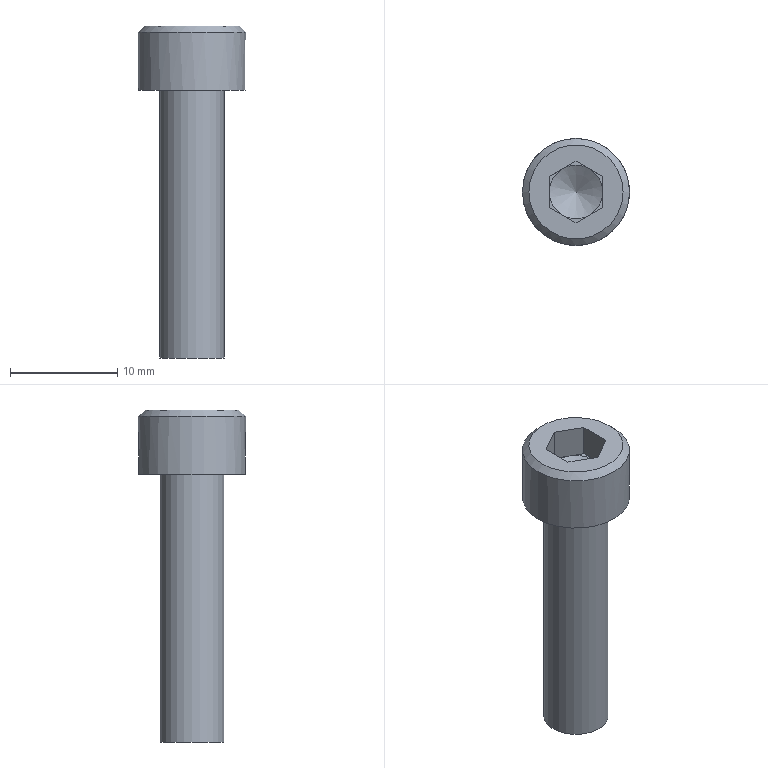Part | NX | features 5003_301_CB6-25 2 | 1 solid | 19 faces | box 10 x 10 x 31 mm | volume 1098 mm3 | plane 15 | cylinder 2 | cone 2 | commonest cylinder face diameters 6 x1 10 x1
STEP:
#1=CARTESIAN_POINT('',(-12.075,-137.,-177.9));
#2=VERTEX_POINT('',#1);
#3=CARTESIAN_POINT('',(-16.475,-137.,-177.9));
#4=DIRECTION('',(0.,0.,-1.));
#5=DIRECTION('',(1.,0.,0.));
#6=AXIS2_PLACEMENT_3D('',#3,#4,#5);
#7=CIRCLE('',#6,4.4);
#8=EDGE_CURVE('',#2,#2,#7,.F.);
#9=ORIENTED_EDGE('',*,*,#8,.T.);
#10=EDGE_LOOP('',(#9));
#11=FACE_BOUND('',#10,.T.);
#12=CARTESIAN_POINT('',(-16.475,-134.113,-177.9));
#13=VERTEX_POINT('',#12);
#14=CARTESIAN_POINT('',(-18.975,-135.557,-177.9));
#15=VERTEX_POINT('',#14);
#16=CARTESIAN_POINT('',(-16.475,-134.113,-177.9));
#17=DIRECTION('',(-0.866,-0.5,0.));
#18=VECTOR('',#17,1000.);
#19=LINE('',#16,#18);
#20=EDGE_CURVE('',#13,#15,#19,.T.);
#21=ORIENTED_EDGE('',*,*,#20,.F.);
#22=CARTESIAN_POINT('',(-13.975,-135.557,-177.9));
#23=VERTEX_POINT('',#22);
#24=CARTESIAN_POINT('',(-13.975,-135.557,-177.9));
#25=DIRECTION('',(-0.866,0.5,0.));
#26=VECTOR('',#25,1000.);
#27=LINE('',#24,#26);
#28=EDGE_CURVE('',#23,#13,#27,.T.);
#29=ORIENTED_EDGE('',*,*,#28,.F.);
#30=CARTESIAN_POINT('',(-13.975,-138.443,-177.9));
#31=VERTEX_POINT('',#30);
#32=CARTESIAN_POINT('',(-13.975,-138.443,-177.9));
#33=DIRECTION('',(0.,1.,0.));
#34=VECTOR('',#33,1000.);
#35=LINE('',#32,#34);
#36=EDGE_CURVE('',#31,#23,#35,.T.);
#37=ORIENTED_EDGE('',*,*,#36,.F.);
#38=CARTESIAN_POINT('',(-16.475,-139.887,-177.9));
#39=VERTEX_POINT('',#38);
#40=CARTESIAN_POINT('',(-16.475,-139.887,-177.9));
#41=DIRECTION('',(0.866,0.5,0.));
#42=VECTOR('',#41,1000.);
#43=LINE('',#40,#42);
#44=EDGE_CURVE('',#39,#31,#43,.T.);
#45=ORIENTED_EDGE('',*,*,#44,.F.);
#46=CARTESIAN_POINT('',(-18.975,-138.443,-177.9));
#47=VERTEX_POINT('',#46);
#48=CARTESIAN_POINT('',(-18.975,-138.443,-177.9));
#49=DIRECTION('',(0.866,-0.5,0.));
#50=VECTOR('',#49,1000.);
#51=LINE('',#48,#50);
#52=EDGE_CURVE('',#47,#39,#51,.T.);
#53=ORIENTED_EDGE('',*,*,#52,.F.);
#54=CARTESIAN_POINT('',(-18.975,-135.557,-177.9));
#55=DIRECTION('',(0.,-1.,0.));
#56=VECTOR('',#55,1000.);
#57=LINE('',#54,#56);
#58=EDGE_CURVE('',#15,#47,#57,.T.);
#59=ORIENTED_EDGE('',*,*,#58,.F.);
#60=EDGE_LOOP('',(#21,#29,#37,#45,#53,#59));
#61=FACE_BOUND('',#60,.T.);
#62=CARTESIAN_POINT('',(-16.475,-142.,-177.9));
#63=DIRECTION('',(0.,0.,-1.));
#64=DIRECTION('',(1.,0.,0.));
#65=AXIS2_PLACEMENT_3D('',#62,#63,#64);
#66=PLANE('',#65);
#67=ADVANCED_FACE('',(#11,#61),#66,.F.);
#68=CARTESIAN_POINT('',(-19.475,-137.,-208.9));
#69=VERTEX_POINT('',#68);
#70=CARTESIAN_POINT('',(-16.475,-137.,-208.9));
#71=DIRECTION('',(0.,0.,1.));
#72=DIRECTION('',(-1.,0.,0.));
#73=AXIS2_PLACEMENT_3D('',#70,#71,#72);
#74=CIRCLE('',#73,3.);
#75=EDGE_CURVE('',#69,#69,#74,.T.);
#76=ORIENTED_EDGE('',*,*,#75,.F.);
#77=EDGE_LOOP('',(#76));
#78=FACE_BOUND('',#77,.T.);
#79=CARTESIAN_POINT('',(-16.475,-137.,-208.9));
#80=DIRECTION('',(0.,0.,1.));
#81=DIRECTION('',(-1.,0.,0.));
#82=AXIS2_PLACEMENT_3D('',#79,#80,#81);
#83=PLANE('',#82);
#84=ADVANCED_FACE('',(#78),#83,.F.);
#85=CARTESIAN_POINT('',(-19.475,-137.,-183.9));
#86=VERTEX_POINT('',#85);
#87=CARTESIAN_POINT('',(-16.475,-137.,-183.9));
#88=DIRECTION('',(0.,0.,1.));
#89=DIRECTION('',(-1.,0.,0.));
#90=AXIS2_PLACEMENT_3D('',#87,#88,#89);
#91=CIRCLE('',#90,3.);
#92=EDGE_CURVE('',#86,#86,#91,.T.);
#93=ORIENTED_EDGE('',*,*,#92,.F.);
#94=EDGE_LOOP('',(#93));
#95=FACE_BOUND('',#94,.T.);
#96=ORIENTED_EDGE('',*,*,#75,.T.);
#97=EDGE_LOOP('',(#96));
#98=FACE_BOUND('',#97,.T.);
#99=CARTESIAN_POINT('',(-16.475,-137.,-177.9));
#100=DIRECTION('',(0.,0.,1.));
#101=DIRECTION('',(-1.,0.,0.));
#102=AXIS2_PLACEMENT_3D('',#99,#100,#101);
#103=CYLINDRICAL_SURFACE('',#102,3.);
#104=ADVANCED_FACE('',(#95,#98),#103,.T.);
#105=CARTESIAN_POINT('',(-21.475,-137.,-183.9));
#106=VERTEX_POINT('',#105);
#107=CARTESIAN_POINT('',(-16.475,-137.,-183.9));
#108=DIRECTION('',(0.,0.,1.));
#109=DIRECTION('',(-1.,0.,0.));
#110=AXIS2_PLACEMENT_3D('',#107,#108,#109);
#111=CIRCLE('',#110,5.);
#112=EDGE_CURVE('',#106,#106,#111,.T.);
#113=ORIENTED_EDGE('',*,*,#112,.F.);
#114=EDGE_LOOP('',(#113));
#115=FACE_BOUND('',#114,.T.);
#116=ORIENTED_EDGE('',*,*,#92,.T.);
#117=EDGE_LOOP('',(#116));
#118=FACE_BOUND('',#117,.T.);
#119=CARTESIAN_POINT('',(-16.475,-140.,-183.9));
#120=DIRECTION('',(0.,0.,1.));
#121=DIRECTION('',(-1.,0.,0.));
#122=AXIS2_PLACEMENT_3D('',#119,#120,#121);
#123=PLANE('',#122);
#124=ADVANCED_FACE('',(#115,#118),#123,.F.);
#125=CARTESIAN_POINT('',(-11.475,-137.,-178.5));
#126=VERTEX_POINT('',#125);
#127=CARTESIAN_POINT('',(-16.475,-137.,-178.5));
#128=DIRECTION('',(0.,0.,-1.));
#129=DIRECTION('',(1.,0.,0.));
#130=AXIS2_PLACEMENT_3D('',#127,#128,#129);
#131=CIRCLE('',#130,5.);
#132=EDGE_CURVE('',#126,#126,#131,.T.);
#133=ORIENTED_EDGE('',*,*,#132,.T.);
#134=EDGE_LOOP('',(#133));
#135=FACE_BOUND('',#134,.T.);
#136=ORIENTED_EDGE('',*,*,#112,.T.);
#137=EDGE_LOOP('',(#136));
#138=FACE_BOUND('',#137,.T.);
#139=CARTESIAN_POINT('',(-16.475,-137.,-177.9));
#140=DIRECTION('',(0.,0.,1.));
#141=DIRECTION('',(-1.,0.,0.));
#142=AXIS2_PLACEMENT_3D('',#139,#140,#141);
#143=CYLINDRICAL_SURFACE('',#142,5.);
#144=ADVANCED_FACE('',(#135,#138),#143,.T.);
#145=ORIENTED_EDGE('',*,*,#132,.F.);
#146=EDGE_LOOP('',(#145));
#147=FACE_BOUND('',#146,.T.);
#148=ORIENTED_EDGE('',*,*,#8,.F.);
#149=EDGE_LOOP('',(#148));
#150=FACE_BOUND('',#149,.T.);
#151=CARTESIAN_POINT('',(-16.475,-137.,-177.9));
#152=DIRECTION('',(0.,0.,-1.));
#153=DIRECTION('',(1.,0.,0.));
#154=AXIS2_PLACEMENT_3D('',#151,#152,#153);
#155=CONICAL_SURFACE('',#154,4.4,0.7854);
#156=ADVANCED_FACE('',(#147,#150),#155,.T.);
#157=CARTESIAN_POINT('',(-13.975,-135.557,-180.9));
#158=VERTEX_POINT('',#157);
#159=CARTESIAN_POINT('',(-15.225,-134.835,-180.9));
#160=VERTEX_POINT('',#159);
#161=CARTESIAN_POINT('',(-13.975,-135.557,-180.9));
#162=DIRECTION('',(-0.866,0.5,0.));
#163=VECTOR('',#162,1000.);
#164=LINE('',#161,#163);
#165=EDGE_CURVE('',#158,#160,#164,.T.);
#166=ORIENTED_EDGE('',*,*,#165,.F.);
#167=CARTESIAN_POINT('',(-13.975,-135.557,-180.9));
#168=DIRECTION('',(0.,0.,1.));
#169=VECTOR('',#168,1000.);
#170=LINE('',#167,#169);
#171=EDGE_CURVE('',#158,#23,#170,.T.);
#172=ORIENTED_EDGE('',*,*,#171,.T.);
#173=ORIENTED_EDGE('',*,*,#28,.T.);
#174=CARTESIAN_POINT('',(-16.475,-134.113,-180.9));
#175=VERTEX_POINT('',#174);
#176=CARTESIAN_POINT('',(-16.475,-134.113,-180.9));
#177=DIRECTION('',(0.,0.,1.));
#178=VECTOR('',#177,1000.);
#179=LINE('',#176,#178);
#180=EDGE_CURVE('',#175,#13,#179,.T.);
#181=ORIENTED_EDGE('',*,*,#180,.F.);
#182=CARTESIAN_POINT('',(-13.975,-135.557,-180.9));
#183=DIRECTION('',(-0.866,0.5,0.));
#184=VECTOR('',#183,1000.);
#185=LINE('',#182,#184);
#186=EDGE_CURVE('',#160,#175,#185,.T.);
#187=ORIENTED_EDGE('',*,*,#186,.F.);
#188=EDGE_LOOP('',(#166,#172,#173,#181,#187));
#189=FACE_BOUND('',#188,.T.);
#190=CARTESIAN_POINT('',(-13.975,-135.557,-180.9));
#191=DIRECTION('',(0.5,0.866,0.));
#192=DIRECTION('',(0.866,-0.5,0.));
#193=AXIS2_PLACEMENT_3D('',#190,#191,#192);
#194=PLANE('',#193);
#195=ADVANCED_FACE('',(#189),#194,.F.);
#196=CARTESIAN_POINT('',(-13.975,-138.443,-180.9));
#197=VERTEX_POINT('',#196);
#198=CARTESIAN_POINT('',(-13.975,-137.,-180.9));
#199=VERTEX_POINT('',#198);
#200=CARTESIAN_POINT('',(-13.975,-138.443,-180.9));
#201=DIRECTION('',(0.,1.,0.));
#202=VECTOR('',#201,1000.);
#203=LINE('',#200,#202);
#204=EDGE_CURVE('',#197,#199,#203,.T.);
#205=ORIENTED_EDGE('',*,*,#204,.F.);
#206=CARTESIAN_POINT('',(-13.975,-138.443,-180.9));
#207=DIRECTION('',(0.,0.,1.));
#208=VECTOR('',#207,1000.);
#209=LINE('',#206,#208);
#210=EDGE_CURVE('',#197,#31,#209,.T.);
#211=ORIENTED_EDGE('',*,*,#210,.T.);
#212=ORIENTED_EDGE('',*,*,#36,.T.);
#213=ORIENTED_EDGE('',*,*,#171,.F.);
#214=CARTESIAN_POINT('',(-13.975,-138.443,-180.9));
#215=DIRECTION('',(0.,1.,0.));
#216=VECTOR('',#215,1000.);
#217=LINE('',#214,#216);
#218=EDGE_CURVE('',#199,#158,#217,.T.);
#219=ORIENTED_EDGE('',*,*,#218,.F.);
#220=EDGE_LOOP('',(#205,#211,#212,#213,#219));
#221=FACE_BOUND('',#220,.T.);
#222=CARTESIAN_POINT('',(-13.975,-138.443,-180.9));
#223=DIRECTION('',(1.,0.,0.));
#224=DIRECTION('',(0.,-1.,0.));
#225=AXIS2_PLACEMENT_3D('',#222,#223,#224);
#226=PLANE('',#225);
#227=ADVANCED_FACE('',(#221),#226,.F.);
#228=CARTESIAN_POINT('',(-16.475,-139.887,-180.9));
#229=VERTEX_POINT('',#228);
#230=CARTESIAN_POINT('',(-15.225,-139.165,-180.9));
#231=VERTEX_POINT('',#230);
#232=CARTESIAN_POINT('',(-16.475,-139.887,-180.9));
#233=DIRECTION('',(0.866,0.5,0.));
#234=VECTOR('',#233,1000.);
#235=LINE('',#232,#234);
#236=EDGE_CURVE('',#229,#231,#235,.T.);
#237=ORIENTED_EDGE('',*,*,#236,.F.);
#238=CARTESIAN_POINT('',(-16.475,-139.887,-180.9));
#239=DIRECTION('',(0.,0.,1.));
#240=VECTOR('',#239,1000.);
#241=LINE('',#238,#240);
#242=EDGE_CURVE('',#229,#39,#241,.T.);
#243=ORIENTED_EDGE('',*,*,#242,.T.);
#244=ORIENTED_EDGE('',*,*,#44,.T.);
#245=ORIENTED_EDGE('',*,*,#210,.F.);
#246=CARTESIAN_POINT('',(-16.475,-139.887,-180.9));
#247=DIRECTION('',(0.866,0.5,0.));
#248=VECTOR('',#247,1000.);
#249=LINE('',#246,#248);
#250=EDGE_CURVE('',#231,#197,#249,.T.);
#251=ORIENTED_EDGE('',*,*,#250,.F.);
#252=EDGE_LOOP('',(#237,#243,#244,#245,#251));
#253=FACE_BOUND('',#252,.T.);
#254=CARTESIAN_POINT('',(-16.475,-139.887,-180.9));
#255=DIRECTION('',(0.5,-0.866,0.));
#256=DIRECTION('',(-0.866,-0.5,0.));
#257=AXIS2_PLACEMENT_3D('',#254,#255,#256);
#258=PLANE('',#257);
#259=ADVANCED_FACE('',(#253),#258,.F.);
#260=CARTESIAN_POINT('',(-18.975,-138.443,-180.9));
#261=VERTEX_POINT('',#260);
#262=CARTESIAN_POINT('',(-17.725,-139.165,-180.9));
#263=VERTEX_POINT('',#262);
#264=CARTESIAN_POINT('',(-18.975,-138.443,-180.9));
#265=DIRECTION('',(0.866,-0.5,0.));
#266=VECTOR('',#265,1000.);
#267=LINE('',#264,#266);
#268=EDGE_CURVE('',#261,#263,#267,.T.);
#269=ORIENTED_EDGE('',*,*,#268,.F.);
#270=CARTESIAN_POINT('',(-18.975,-138.443,-180.9));
#271=DIRECTION('',(0.,0.,1.));
#272=VECTOR('',#271,1000.);
#273=LINE('',#270,#272);
#274=EDGE_CURVE('',#261,#47,#273,.T.);
#275=ORIENTED_EDGE('',*,*,#274,.T.);
#276=ORIENTED_EDGE('',*,*,#52,.T.);
#277=ORIENTED_EDGE('',*,*,#242,.F.);
#278=CARTESIAN_POINT('',(-18.975,-138.443,-180.9));
#279=DIRECTION('',(0.866,-0.5,0.));
#280=VECTOR('',#279,1000.);
#281=LINE('',#278,#280);
#282=EDGE_CURVE('',#263,#229,#281,.T.);
#283=ORIENTED_EDGE('',*,*,#282,.F.);
#284=EDGE_LOOP('',(#269,#275,#276,#277,#283));
#285=FACE_BOUND('',#284,.T.);
#286=CARTESIAN_POINT('',(-18.975,-138.443,-180.9));
#287=DIRECTION('',(-0.5,-0.866,0.));
#288=DIRECTION('',(-0.866,0.5,0.));
#289=AXIS2_PLACEMENT_3D('',#286,#287,#288);
#290=PLANE('',#289);
#291=ADVANCED_FACE('',(#285),#290,.F.);
#292=CARTESIAN_POINT('',(-18.975,-135.557,-180.9));
#293=VERTEX_POINT('',#292);
#294=CARTESIAN_POINT('',(-18.975,-137.,-180.9));
#295=VERTEX_POINT('',#294);
#296=CARTESIAN_POINT('',(-18.975,-135.557,-180.9));
#297=DIRECTION('',(0.,-1.,0.));
#298=VECTOR('',#297,1000.);
#299=LINE('',#296,#298);
#300=EDGE_CURVE('',#293,#295,#299,.T.);
#301=ORIENTED_EDGE('',*,*,#300,.F.);
#302=CARTESIAN_POINT('',(-18.975,-135.557,-180.9));
#303=DIRECTION('',(0.,0.,1.));
#304=VECTOR('',#303,1000.);
#305=LINE('',#302,#304);
#306=EDGE_CURVE('',#293,#15,#305,.T.);
#307=ORIENTED_EDGE('',*,*,#306,.T.);
#308=ORIENTED_EDGE('',*,*,#58,.T.);
#309=ORIENTED_EDGE('',*,*,#274,.F.);
#310=CARTESIAN_POINT('',(-18.975,-135.557,-180.9));
#311=DIRECTION('',(0.,-1.,0.));
#312=VECTOR('',#311,1000.);
#313=LINE('',#310,#312);
#314=EDGE_CURVE('',#295,#261,#313,.T.);
#315=ORIENTED_EDGE('',*,*,#314,.F.);
#316=EDGE_LOOP('',(#301,#307,#308,#309,#315));
#317=FACE_BOUND('',#316,.T.);
#318=CARTESIAN_POINT('',(-18.975,-135.557,-180.9));
#319=DIRECTION('',(-1.,0.,0.));
#320=DIRECTION('',(0.,0.,-1.));
#321=AXIS2_PLACEMENT_3D('',#318,#319,#320);
#322=PLANE('',#321);
#323=ADVANCED_FACE('',(#317),#322,.F.);
#324=CARTESIAN_POINT('',(-17.725,-134.835,-180.9));
#325=VERTEX_POINT('',#324);
#326=CARTESIAN_POINT('',(-16.475,-134.113,-180.9));
#327=DIRECTION('',(-0.866,-0.5,0.));
#328=VECTOR('',#327,1000.);
#329=LINE('',#326,#328);
#330=EDGE_CURVE('',#175,#325,#329,.T.);
#331=ORIENTED_EDGE('',*,*,#330,.F.);
#332=ORIENTED_EDGE('',*,*,#180,.T.);
#333=ORIENTED_EDGE('',*,*,#20,.T.);
#334=ORIENTED_EDGE('',*,*,#306,.F.);
#335=CARTESIAN_POINT('',(-16.475,-134.113,-180.9));
#336=DIRECTION('',(-0.866,-0.5,0.));
#337=VECTOR('',#336,1000.);
#338=LINE('',#335,#337);
#339=EDGE_CURVE('',#325,#293,#338,.T.);
#340=ORIENTED_EDGE('',*,*,#339,.F.);
#341=EDGE_LOOP('',(#331,#332,#333,#334,#340));
#342=FACE_BOUND('',#341,.T.);
#343=CARTESIAN_POINT('',(-16.475,-134.113,-180.9));
#344=DIRECTION('',(-0.5,0.866,0.));
#345=DIRECTION('',(0.866,0.5,0.));
#346=AXIS2_PLACEMENT_3D('',#343,#344,#345);
#347=PLANE('',#346);
#348=ADVANCED_FACE('',(#342),#347,.F.);
#349=ORIENTED_EDGE('',*,*,#314,.T.);
#350=ORIENTED_EDGE('',*,*,#268,.T.);
#351=CARTESIAN_POINT('',(-16.475,-137.,-180.9));
#352=DIRECTION('',(0.,0.,1.));
#353=DIRECTION('',(0.,1.,0.));
#354=AXIS2_PLACEMENT_3D('',#351,#352,#353);
#355=CIRCLE('',#354,2.5);
#356=EDGE_CURVE('',#295,#263,#355,.T.);
#357=ORIENTED_EDGE('',*,*,#356,.F.);
#358=EDGE_LOOP('',(#349,#350,#357));
#359=FACE_BOUND('',#358,.T.);
#360=CARTESIAN_POINT('',(-16.475,-137.,-180.9));
#361=DIRECTION('',(0.,0.,1.));
#362=DIRECTION('',(-1.,0.,0.));
#363=AXIS2_PLACEMENT_3D('',#360,#361,#362);
#364=PLANE('',#363);
#365=ADVANCED_FACE('',(#359),#364,.T.);
#366=ORIENTED_EDGE('',*,*,#282,.T.);
#367=ORIENTED_EDGE('',*,*,#236,.T.);
#368=CARTESIAN_POINT('',(-16.475,-137.,-180.9));
#369=DIRECTION('',(0.,0.,1.));
#370=DIRECTION('',(0.,1.,0.));
#371=AXIS2_PLACEMENT_3D('',#368,#369,#370);
#372=CIRCLE('',#371,2.5);
#373=EDGE_CURVE('',#263,#231,#372,.T.);
#374=ORIENTED_EDGE('',*,*,#373,.F.);
#375=EDGE_LOOP('',(#366,#367,#374));
#376=FACE_BOUND('',#375,.T.);
#377=CARTESIAN_POINT('',(-16.475,-137.,-180.9));
#378=DIRECTION('',(0.,0.,1.));
#379=DIRECTION('',(-1.,0.,0.));
#380=AXIS2_PLACEMENT_3D('',#377,#378,#379);
#381=PLANE('',#380);
#382=ADVANCED_FACE('',(#376),#381,.T.);
#383=ORIENTED_EDGE('',*,*,#250,.T.);
#384=ORIENTED_EDGE('',*,*,#204,.T.);
#385=CARTESIAN_POINT('',(-16.475,-137.,-180.9));
#386=DIRECTION('',(0.,0.,1.));
#387=DIRECTION('',(0.,1.,0.));
#388=AXIS2_PLACEMENT_3D('',#385,#386,#387);
#389=CIRCLE('',#388,2.5);
#390=EDGE_CURVE('',#231,#199,#389,.T.);
#391=ORIENTED_EDGE('',*,*,#390,.F.);
#392=EDGE_LOOP('',(#383,#384,#391));
#393=FACE_BOUND('',#392,.T.);
#394=CARTESIAN_POINT('',(-16.475,-137.,-180.9));
#395=DIRECTION('',(0.,0.,1.));
#396=DIRECTION('',(-1.,0.,0.));
#397=AXIS2_PLACEMENT_3D('',#394,#395,#396);
#398=PLANE('',#397);
#399=ADVANCED_FACE('',(#393),#398,.T.);
#400=ORIENTED_EDGE('',*,*,#218,.T.);
#401=ORIENTED_EDGE('',*,*,#165,.T.);
#402=CARTESIAN_POINT('',(-16.475,-137.,-180.9));
#403=DIRECTION('',(0.,0.,1.));
#404=DIRECTION('',(0.,1.,0.));
#405=AXIS2_PLACEMENT_3D('',#402,#403,#404);
#406=CIRCLE('',#405,2.5);
#407=EDGE_CURVE('',#199,#160,#406,.T.);
#408=ORIENTED_EDGE('',*,*,#407,.F.);
#409=EDGE_LOOP('',(#400,#401,#408));
#410=FACE_BOUND('',#409,.T.);
#411=CARTESIAN_POINT('',(-16.475,-137.,-180.9));
#412=DIRECTION('',(0.,0.,1.));
#413=DIRECTION('',(-1.,0.,0.));
#414=AXIS2_PLACEMENT_3D('',#411,#412,#413);
#415=PLANE('',#414);
#416=ADVANCED_FACE('',(#410),#415,.T.);
#417=ORIENTED_EDGE('',*,*,#186,.T.);
#418=ORIENTED_EDGE('',*,*,#330,.T.);
#419=CARTESIAN_POINT('',(-16.475,-137.,-180.9));
#420=DIRECTION('',(0.,0.,1.));
#421=DIRECTION('',(0.,1.,0.));
#422=AXIS2_PLACEMENT_3D('',#419,#420,#421);
#423=CIRCLE('',#422,2.5);
#424=EDGE_CURVE('',#160,#325,#423,.T.);
#425=ORIENTED_EDGE('',*,*,#424,.F.);
#426=EDGE_LOOP('',(#417,#418,#425));
#427=FACE_BOUND('',#426,.T.);
#428=CARTESIAN_POINT('',(-16.475,-137.,-180.9));
#429=DIRECTION('',(0.,0.,1.));
#430=DIRECTION('',(-1.,0.,0.));
#431=AXIS2_PLACEMENT_3D('',#428,#429,#430);
#432=PLANE('',#431);
#433=ADVANCED_FACE('',(#427),#432,.T.);
#434=ORIENTED_EDGE('',*,*,#339,.T.);
#435=ORIENTED_EDGE('',*,*,#300,.T.);
#436=CARTESIAN_POINT('',(-16.475,-137.,-180.9));
#437=DIRECTION('',(0.,0.,1.));
#438=DIRECTION('',(0.,1.,0.));
#439=AXIS2_PLACEMENT_3D('',#436,#437,#438);
#440=CIRCLE('',#439,2.5);
#441=EDGE_CURVE('',#325,#295,#440,.T.);
#442=ORIENTED_EDGE('',*,*,#441,.F.);
#443=EDGE_LOOP('',(#434,#435,#442));
#444=FACE_BOUND('',#443,.T.);
#445=CARTESIAN_POINT('',(-16.475,-137.,-180.9));
#446=DIRECTION('',(0.,0.,1.));
#447=DIRECTION('',(-1.,0.,0.));
#448=AXIS2_PLACEMENT_3D('',#445,#446,#447);
#449=PLANE('',#448);
#450=ADVANCED_FACE('',(#444),#449,.T.);
#451=ORIENTED_EDGE('',*,*,#441,.T.);
#452=ORIENTED_EDGE('',*,*,#356,.T.);
#453=ORIENTED_EDGE('',*,*,#373,.T.);
#454=ORIENTED_EDGE('',*,*,#390,.T.);
#455=ORIENTED_EDGE('',*,*,#407,.T.);
#456=ORIENTED_EDGE('',*,*,#424,.T.);
#457=EDGE_LOOP('',(#451,#452,#453,#454,#455,#456));
#458=FACE_BOUND('',#457,.T.);
#459=CARTESIAN_POINT('',(-16.475,-137.,-182.402));
#460=VERTEX_POINT('',#459);
#461=VERTEX_LOOP('',#460);
#462=FACE_BOUND('',#461,.T.);
#463=CARTESIAN_POINT('',(-16.475,-137.,-182.402));
#464=DIRECTION('',(0.,0.,1.));
#465=DIRECTION('',(0.,1.,0.));
#466=AXIS2_PLACEMENT_3D('',#463,#464,#465);
#467=CONICAL_SURFACE('',#466,0.,1.03);
#468=ADVANCED_FACE('',(#458,#462),#467,.F.);
#469=CLOSED_SHELL('',(#67,#84,#104,#124,#144,#156,#195,#227,#259,#291,#323,#348,#365,#382,#399,#416,#433,#450,#468));
#470=MANIFOLD_SOLID_BREP('',#469);
#471=(LENGTH_UNIT()NAMED_UNIT(*)SI_UNIT(.MILLI.,.METRE.));
#472=UNCERTAINTY_MEASURE_WITH_UNIT(LENGTH_MEASURE(0.00001),#471,'','');
#473=(NAMED_UNIT(*)PLANE_ANGLE_UNIT()SI_UNIT($,.RADIAN.));
#474=(NAMED_UNIT(*)SI_UNIT($,.STERADIAN.)SOLID_ANGLE_UNIT());
#475=(GEOMETRIC_REPRESENTATION_CONTEXT(3)GLOBAL_UNCERTAINTY_ASSIGNED_CONTEXT((#472))GLOBAL_UNIT_ASSIGNED_CONTEXT((#471,#473,#474))REPRESENTATION_CONTEXT('',''));
#476=ADVANCED_BREP_SHAPE_REPRESENTATION('',(#470),#475);